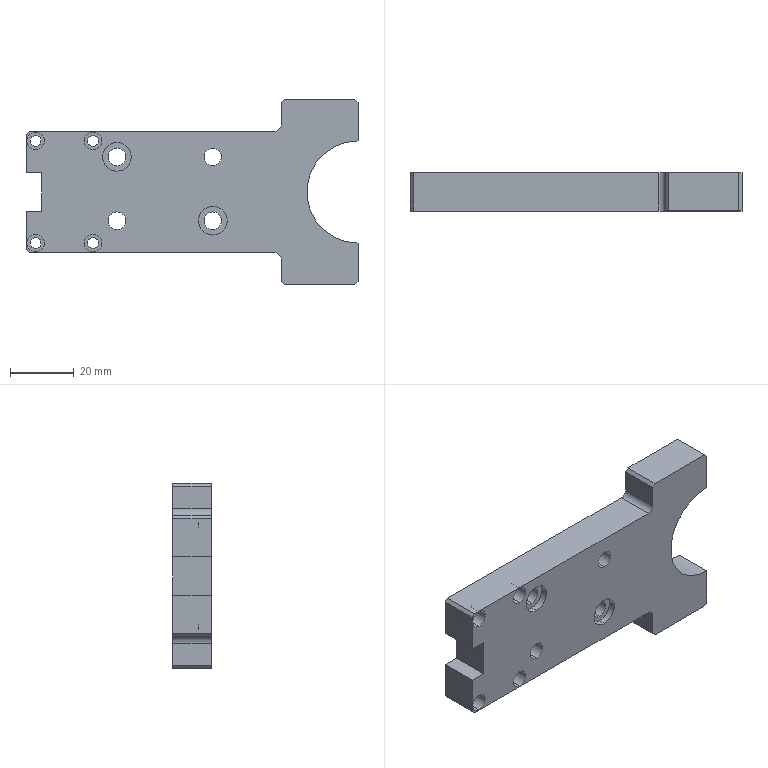Part | SolidWorks | features ICE 6, HoleWzd 3, Chamfer 1, Extrusion 1, Fillet 1 | 1 solid | 84 faces | box 104 x 12 x 58 mm | volume 44083 mm3 | cylinder 47 | plane 33 | cone 4 | commonest cylinder face diameters 5.5 x16 3.4 x8 10 x8 3.3 x4 5 x4 9 x4